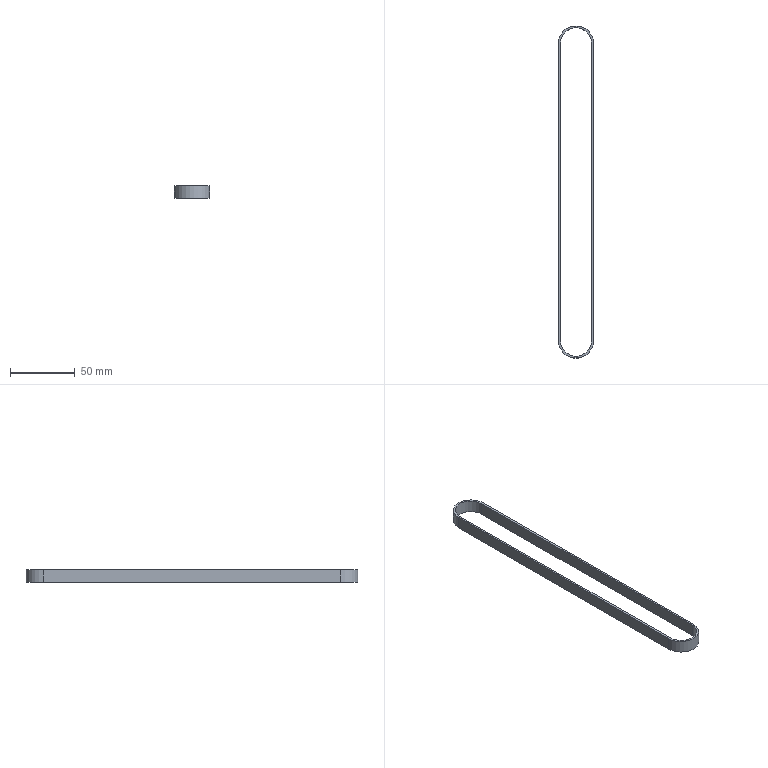Part | STEP file | KRBT-S3M-100- 179 | 1 solid | 10 faces | box 27.07 x 256.613 x 10 mm | volume 8091 mm3 | plane 6 | cylinder 4 | commonest cylinder face diameters 24.07 x2 27.07 x2
STEP:
#1=CARTESIAN_POINT('',(-8.535,4.307,5.));
#2=VERTEX_POINT('',#1);
#3=CARTESIAN_POINT('',(18.535,4.307,5.));
#4=VERTEX_POINT('',#3);
#5=CARTESIAN_POINT('',(5.,4.307,5.));
#6=DIRECTION('',(0.,0.,1.));
#7=DIRECTION('',(-1.,0.,0.));
#8=AXIS2_PLACEMENT_3D('',#5,#6,#7);
#9=CIRCLE('',#8,13.535);
#10=EDGE_CURVE('',#2,#4,#9,.T.);
#11=ORIENTED_EDGE('',*,*,#10,.T.);
#12=CARTESIAN_POINT('',(18.535,233.85,5.));
#13=VERTEX_POINT('',#12);
#14=CARTESIAN_POINT('',(18.535,4.307,5.));
#15=DIRECTION('',(0.,1.,0.));
#16=VECTOR('',#15,1000.);
#17=LINE('',#14,#16);
#18=EDGE_CURVE('',#4,#13,#17,.T.);
#19=ORIENTED_EDGE('',*,*,#18,.T.);
#20=CARTESIAN_POINT('',(-8.535,233.85,5.));
#21=VERTEX_POINT('',#20);
#22=CARTESIAN_POINT('',(5.,233.85,5.));
#23=DIRECTION('',(0.,0.,1.));
#24=DIRECTION('',(-1.,0.,0.));
#25=AXIS2_PLACEMENT_3D('',#22,#23,#24);
#26=CIRCLE('',#25,13.535);
#27=EDGE_CURVE('',#13,#21,#26,.T.);
#28=ORIENTED_EDGE('',*,*,#27,.T.);
#29=CARTESIAN_POINT('',(-8.535,4.307,5.));
#30=DIRECTION('',(0.,-1.,0.));
#31=VECTOR('',#30,1000.);
#32=LINE('',#29,#31);
#33=EDGE_CURVE('',#21,#2,#32,.T.);
#34=ORIENTED_EDGE('',*,*,#33,.T.);
#35=EDGE_LOOP('',(#11,#19,#28,#34));
#36=FACE_OUTER_BOUND('',#35,.T.);
#37=CARTESIAN_POINT('',(-7.035,4.307,5.));
#38=VERTEX_POINT('',#37);
#39=CARTESIAN_POINT('',(17.035,4.307,5.));
#40=VERTEX_POINT('',#39);
#41=CARTESIAN_POINT('',(5.,4.307,5.));
#42=DIRECTION('',(0.,0.,1.));
#43=DIRECTION('',(-1.,0.,0.));
#44=AXIS2_PLACEMENT_3D('',#41,#42,#43);
#45=CIRCLE('',#44,12.035);
#46=EDGE_CURVE('',#38,#40,#45,.T.);
#47=ORIENTED_EDGE('',*,*,#46,.F.);
#48=CARTESIAN_POINT('',(-7.035,233.85,5.));
#49=VERTEX_POINT('',#48);
#50=CARTESIAN_POINT('',(-7.035,4.307,5.));
#51=DIRECTION('',(0.,-1.,0.));
#52=VECTOR('',#51,1000.);
#53=LINE('',#50,#52);
#54=EDGE_CURVE('',#49,#38,#53,.T.);
#55=ORIENTED_EDGE('',*,*,#54,.F.);
#56=CARTESIAN_POINT('',(17.035,233.85,5.));
#57=VERTEX_POINT('',#56);
#58=CARTESIAN_POINT('',(5.,233.85,5.));
#59=DIRECTION('',(0.,0.,1.));
#60=DIRECTION('',(-1.,0.,0.));
#61=AXIS2_PLACEMENT_3D('',#58,#59,#60);
#62=CIRCLE('',#61,12.035);
#63=EDGE_CURVE('',#57,#49,#62,.T.);
#64=ORIENTED_EDGE('',*,*,#63,.F.);
#65=CARTESIAN_POINT('',(17.035,233.85,5.));
#66=DIRECTION('',(0.,1.,0.));
#67=VECTOR('',#66,1000.);
#68=LINE('',#65,#67);
#69=EDGE_CURVE('',#40,#57,#68,.T.);
#70=ORIENTED_EDGE('',*,*,#69,.F.);
#71=EDGE_LOOP('',(#47,#55,#64,#70));
#72=FACE_BOUND('',#71,.T.);
#73=CARTESIAN_POINT('',(5.,4.307,5.));
#74=DIRECTION('',(0.,0.,-1.));
#75=DIRECTION('',(-1.,0.,0.));
#76=AXIS2_PLACEMENT_3D('',#73,#74,#75);
#77=PLANE('',#76);
#78=ADVANCED_FACE('',(#36,#72),#77,.F.);
#79=CARTESIAN_POINT('',(-8.535,4.307,-5.));
#80=VERTEX_POINT('',#79);
#81=CARTESIAN_POINT('',(18.535,4.307,-5.));
#82=VERTEX_POINT('',#81);
#83=CARTESIAN_POINT('',(5.,4.307,-5.));
#84=DIRECTION('',(0.,0.,1.));
#85=DIRECTION('',(-1.,0.,0.));
#86=AXIS2_PLACEMENT_3D('',#83,#84,#85);
#87=CIRCLE('',#86,13.535);
#88=EDGE_CURVE('',#80,#82,#87,.T.);
#89=ORIENTED_EDGE('',*,*,#88,.F.);
#90=CARTESIAN_POINT('',(-8.535,233.85,-5.));
#91=VERTEX_POINT('',#90);
#92=CARTESIAN_POINT('',(-8.535,4.307,-5.));
#93=DIRECTION('',(0.,-1.,0.));
#94=VECTOR('',#93,1000.);
#95=LINE('',#92,#94);
#96=EDGE_CURVE('',#91,#80,#95,.T.);
#97=ORIENTED_EDGE('',*,*,#96,.F.);
#98=CARTESIAN_POINT('',(18.535,233.85,-5.));
#99=VERTEX_POINT('',#98);
#100=CARTESIAN_POINT('',(5.,233.85,-5.));
#101=DIRECTION('',(0.,0.,1.));
#102=DIRECTION('',(-1.,0.,0.));
#103=AXIS2_PLACEMENT_3D('',#100,#101,#102);
#104=CIRCLE('',#103,13.535);
#105=EDGE_CURVE('',#99,#91,#104,.T.);
#106=ORIENTED_EDGE('',*,*,#105,.F.);
#107=CARTESIAN_POINT('',(18.535,4.307,-5.));
#108=DIRECTION('',(0.,1.,0.));
#109=VECTOR('',#108,1000.);
#110=LINE('',#107,#109);
#111=EDGE_CURVE('',#82,#99,#110,.T.);
#112=ORIENTED_EDGE('',*,*,#111,.F.);
#113=EDGE_LOOP('',(#89,#97,#106,#112));
#114=FACE_OUTER_BOUND('',#113,.T.);
#115=CARTESIAN_POINT('',(-7.035,233.85,-5.));
#116=VERTEX_POINT('',#115);
#117=CARTESIAN_POINT('',(-7.035,4.307,-5.));
#118=VERTEX_POINT('',#117);
#119=CARTESIAN_POINT('',(-7.035,4.307,-5.));
#120=DIRECTION('',(0.,-1.,0.));
#121=VECTOR('',#120,1000.);
#122=LINE('',#119,#121);
#123=EDGE_CURVE('',#116,#118,#122,.T.);
#124=ORIENTED_EDGE('',*,*,#123,.T.);
#125=CARTESIAN_POINT('',(17.035,4.307,-5.));
#126=VERTEX_POINT('',#125);
#127=CARTESIAN_POINT('',(5.,4.307,-5.));
#128=DIRECTION('',(0.,0.,1.));
#129=DIRECTION('',(-1.,0.,0.));
#130=AXIS2_PLACEMENT_3D('',#127,#128,#129);
#131=CIRCLE('',#130,12.035);
#132=EDGE_CURVE('',#118,#126,#131,.T.);
#133=ORIENTED_EDGE('',*,*,#132,.T.);
#134=CARTESIAN_POINT('',(17.035,233.85,-5.));
#135=VERTEX_POINT('',#134);
#136=CARTESIAN_POINT('',(17.035,233.85,-5.));
#137=DIRECTION('',(0.,1.,0.));
#138=VECTOR('',#137,1000.);
#139=LINE('',#136,#138);
#140=EDGE_CURVE('',#126,#135,#139,.T.);
#141=ORIENTED_EDGE('',*,*,#140,.T.);
#142=CARTESIAN_POINT('',(5.,233.85,-5.));
#143=DIRECTION('',(0.,0.,1.));
#144=DIRECTION('',(-1.,0.,0.));
#145=AXIS2_PLACEMENT_3D('',#142,#143,#144);
#146=CIRCLE('',#145,12.035);
#147=EDGE_CURVE('',#135,#116,#146,.T.);
#148=ORIENTED_EDGE('',*,*,#147,.T.);
#149=EDGE_LOOP('',(#124,#133,#141,#148));
#150=FACE_BOUND('',#149,.T.);
#151=CARTESIAN_POINT('',(5.,4.307,-5.));
#152=DIRECTION('',(0.,0.,-1.));
#153=DIRECTION('',(-1.,0.,0.));
#154=AXIS2_PLACEMENT_3D('',#151,#152,#153);
#155=PLANE('',#154);
#156=ADVANCED_FACE('',(#114,#150),#155,.T.);
#157=ORIENTED_EDGE('',*,*,#88,.T.);
#158=CARTESIAN_POINT('',(18.535,4.307,5.));
#159=DIRECTION('',(0.,0.,-1.));
#160=VECTOR('',#159,1000.);
#161=LINE('',#158,#160);
#162=EDGE_CURVE('',#4,#82,#161,.T.);
#163=ORIENTED_EDGE('',*,*,#162,.F.);
#164=ORIENTED_EDGE('',*,*,#10,.F.);
#165=CARTESIAN_POINT('',(-8.535,4.307,5.));
#166=DIRECTION('',(0.,0.,-1.));
#167=VECTOR('',#166,1000.);
#168=LINE('',#165,#167);
#169=EDGE_CURVE('',#2,#80,#168,.T.);
#170=ORIENTED_EDGE('',*,*,#169,.T.);
#171=EDGE_LOOP('',(#157,#163,#164,#170));
#172=FACE_OUTER_BOUND('',#171,.T.);
#173=CARTESIAN_POINT('',(5.,4.307,5.));
#174=DIRECTION('',(0.,0.,-1.));
#175=DIRECTION('',(-1.,0.,0.));
#176=AXIS2_PLACEMENT_3D('',#173,#174,#175);
#177=CYLINDRICAL_SURFACE('',#176,13.535);
#178=ADVANCED_FACE('',(#172),#177,.T.);
#179=ORIENTED_EDGE('',*,*,#111,.T.);
#180=CARTESIAN_POINT('',(18.535,233.85,5.));
#181=DIRECTION('',(0.,0.,-1.));
#182=VECTOR('',#181,1000.);
#183=LINE('',#180,#182);
#184=EDGE_CURVE('',#13,#99,#183,.T.);
#185=ORIENTED_EDGE('',*,*,#184,.F.);
#186=ORIENTED_EDGE('',*,*,#18,.F.);
#187=ORIENTED_EDGE('',*,*,#162,.T.);
#188=EDGE_LOOP('',(#179,#185,#186,#187));
#189=FACE_OUTER_BOUND('',#188,.T.);
#190=CARTESIAN_POINT('',(18.535,4.307,5.));
#191=DIRECTION('',(-1.,0.,0.));
#192=DIRECTION('',(0.,-1.,0.));
#193=AXIS2_PLACEMENT_3D('',#190,#191,#192);
#194=PLANE('',#193);
#195=ADVANCED_FACE('',(#189),#194,.F.);
#196=ORIENTED_EDGE('',*,*,#105,.T.);
#197=CARTESIAN_POINT('',(-8.535,233.85,5.));
#198=DIRECTION('',(0.,0.,-1.));
#199=VECTOR('',#198,1000.);
#200=LINE('',#197,#199);
#201=EDGE_CURVE('',#21,#91,#200,.T.);
#202=ORIENTED_EDGE('',*,*,#201,.F.);
#203=ORIENTED_EDGE('',*,*,#27,.F.);
#204=ORIENTED_EDGE('',*,*,#184,.T.);
#205=EDGE_LOOP('',(#196,#202,#203,#204));
#206=FACE_OUTER_BOUND('',#205,.T.);
#207=CARTESIAN_POINT('',(5.,233.85,5.));
#208=DIRECTION('',(0.,0.,-1.));
#209=DIRECTION('',(-1.,0.,0.));
#210=AXIS2_PLACEMENT_3D('',#207,#208,#209);
#211=CYLINDRICAL_SURFACE('',#210,13.535);
#212=ADVANCED_FACE('',(#206),#211,.T.);
#213=ORIENTED_EDGE('',*,*,#96,.T.);
#214=ORIENTED_EDGE('',*,*,#169,.F.);
#215=ORIENTED_EDGE('',*,*,#33,.F.);
#216=ORIENTED_EDGE('',*,*,#201,.T.);
#217=EDGE_LOOP('',(#213,#214,#215,#216));
#218=FACE_OUTER_BOUND('',#217,.T.);
#219=CARTESIAN_POINT('',(-8.535,4.307,5.));
#220=DIRECTION('',(1.,0.,0.));
#221=DIRECTION('',(0.,1.,0.));
#222=AXIS2_PLACEMENT_3D('',#219,#220,#221);
#223=PLANE('',#222);
#224=ADVANCED_FACE('',(#218),#223,.F.);
#225=ORIENTED_EDGE('',*,*,#132,.F.);
#226=CARTESIAN_POINT('',(-7.035,4.307,5.));
#227=DIRECTION('',(0.,0.,-1.));
#228=VECTOR('',#227,1000.);
#229=LINE('',#226,#228);
#230=EDGE_CURVE('',#38,#118,#229,.T.);
#231=ORIENTED_EDGE('',*,*,#230,.F.);
#232=ORIENTED_EDGE('',*,*,#46,.T.);
#233=CARTESIAN_POINT('',(17.035,4.307,5.));
#234=DIRECTION('',(0.,0.,-1.));
#235=VECTOR('',#234,1000.);
#236=LINE('',#233,#235);
#237=EDGE_CURVE('',#40,#126,#236,.T.);
#238=ORIENTED_EDGE('',*,*,#237,.T.);
#239=EDGE_LOOP('',(#225,#231,#232,#238));
#240=FACE_OUTER_BOUND('',#239,.T.);
#241=CARTESIAN_POINT('',(5.,4.307,5.));
#242=DIRECTION('',(0.,0.,-1.));
#243=DIRECTION('',(-1.,0.,0.));
#244=AXIS2_PLACEMENT_3D('',#241,#242,#243);
#245=CYLINDRICAL_SURFACE('',#244,12.035);
#246=ADVANCED_FACE('',(#240),#245,.F.);
#247=ORIENTED_EDGE('',*,*,#140,.F.);
#248=ORIENTED_EDGE('',*,*,#237,.F.);
#249=ORIENTED_EDGE('',*,*,#69,.T.);
#250=CARTESIAN_POINT('',(17.035,233.85,5.));
#251=DIRECTION('',(0.,0.,-1.));
#252=VECTOR('',#251,1000.);
#253=LINE('',#250,#252);
#254=EDGE_CURVE('',#57,#135,#253,.T.);
#255=ORIENTED_EDGE('',*,*,#254,.T.);
#256=EDGE_LOOP('',(#247,#248,#249,#255));
#257=FACE_OUTER_BOUND('',#256,.T.);
#258=CARTESIAN_POINT('',(17.035,233.85,5.));
#259=DIRECTION('',(-1.,0.,0.));
#260=DIRECTION('',(0.,-1.,0.));
#261=AXIS2_PLACEMENT_3D('',#258,#259,#260);
#262=PLANE('',#261);
#263=ADVANCED_FACE('',(#257),#262,.T.);
#264=ORIENTED_EDGE('',*,*,#147,.F.);
#265=ORIENTED_EDGE('',*,*,#254,.F.);
#266=ORIENTED_EDGE('',*,*,#63,.T.);
#267=CARTESIAN_POINT('',(-7.035,233.85,5.));
#268=DIRECTION('',(0.,0.,-1.));
#269=VECTOR('',#268,1000.);
#270=LINE('',#267,#269);
#271=EDGE_CURVE('',#49,#116,#270,.T.);
#272=ORIENTED_EDGE('',*,*,#271,.T.);
#273=EDGE_LOOP('',(#264,#265,#266,#272));
#274=FACE_OUTER_BOUND('',#273,.T.);
#275=CARTESIAN_POINT('',(5.,233.85,5.));
#276=DIRECTION('',(0.,0.,-1.));
#277=DIRECTION('',(-1.,0.,0.));
#278=AXIS2_PLACEMENT_3D('',#275,#276,#277);
#279=CYLINDRICAL_SURFACE('',#278,12.035);
#280=ADVANCED_FACE('',(#274),#279,.F.);
#281=ORIENTED_EDGE('',*,*,#123,.F.);
#282=ORIENTED_EDGE('',*,*,#271,.F.);
#283=ORIENTED_EDGE('',*,*,#54,.T.);
#284=ORIENTED_EDGE('',*,*,#230,.T.);
#285=EDGE_LOOP('',(#281,#282,#283,#284));
#286=FACE_OUTER_BOUND('',#285,.T.);
#287=CARTESIAN_POINT('',(-7.035,4.307,5.));
#288=DIRECTION('',(1.,0.,0.));
#289=DIRECTION('',(0.,1.,0.));
#290=AXIS2_PLACEMENT_3D('',#287,#288,#289);
#291=PLANE('',#290);
#292=ADVANCED_FACE('',(#286),#291,.T.);
#293=CLOSED_SHELL('',(#78,#156,#178,#195,#212,#224,#246,#263,#280,#292));
#294=MANIFOLD_SOLID_BREP('',#293);
#295=CARTESIAN_POINT('',(0.,0.,0.));
#296=DIRECTION('',(0.,0.,1.));
#297=DIRECTION('',(1.,0.,0.));
#298=AXIS2_PLACEMENT_3D('',#295,#296,#297);
#299=(LENGTH_UNIT()NAMED_UNIT(*)SI_UNIT(.MILLI.,.METRE.));
#300=UNCERTAINTY_MEASURE_WITH_UNIT(LENGTH_MEASURE(0.00001),#299,'','');
#301=(NAMED_UNIT(*)PLANE_ANGLE_UNIT()SI_UNIT($,.RADIAN.));
#302=(NAMED_UNIT(*)SI_UNIT($,.STERADIAN.)SOLID_ANGLE_UNIT());
#303=(GEOMETRIC_REPRESENTATION_CONTEXT(3)GLOBAL_UNCERTAINTY_ASSIGNED_CONTEXT((#300))GLOBAL_UNIT_ASSIGNED_CONTEXT((#299,#301,#302))REPRESENTATION_CONTEXT('',''));
#304=ADVANCED_BREP_SHAPE_REPRESENTATION('',(#294,#298),#303);